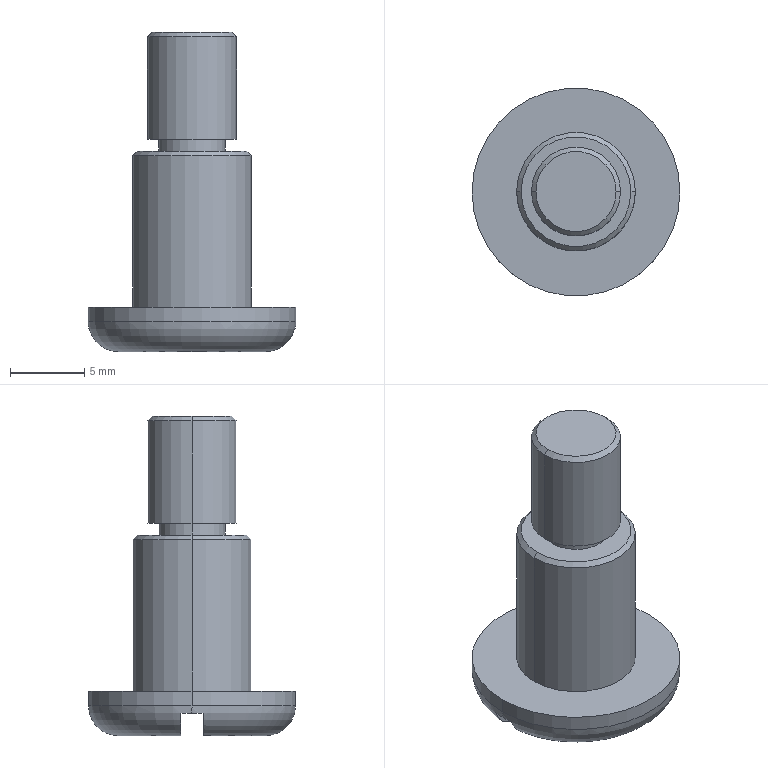Part | SolidWorks | features ICE 4, Chamfer 1, Extrusion 1, Fillet 1 | 1 solid | 23 faces | box 14 x 14 x 21.5 mm | volume 1140 mm3 | plane 9 | cylinder 8 | cone 4 | torus 2 | commonest cylinder face diameters 4.5 x2 6 x2 8 x2 14 x2
STEP:
#1=CARTESIAN_POINT('',(2.7,0.,21.5));
#2=VERTEX_POINT('',#1);
#3=CARTESIAN_POINT('',(-2.7,0.,21.5));
#4=VERTEX_POINT('',#3);
#5=CARTESIAN_POINT('',(0.,0.,21.5));
#6=DIRECTION('',(0.,0.,1.));
#7=DIRECTION('',(1.,0.,0.));
#8=AXIS2_PLACEMENT_3D('',#5,#6,#7);
#9=CIRCLE('',#8,2.7);
#10=EDGE_CURVE('',#2,#4,#9,.T.);
#11=ORIENTED_EDGE('',*,*,#10,.F.);
#12=CARTESIAN_POINT('',(3.,0.,21.2));
#13=VERTEX_POINT('',#12);
#14=CARTESIAN_POINT('',(2.7,0.,21.5));
#15=DIRECTION('',(0.7071,0.,-0.7071));
#16=VECTOR('',#15,1000.);
#17=LINE('',#14,#16);
#18=EDGE_CURVE('',#2,#13,#17,.T.);
#19=ORIENTED_EDGE('',*,*,#18,.T.);
#20=CARTESIAN_POINT('',(-3.,0.,21.2));
#21=VERTEX_POINT('',#20);
#22=CARTESIAN_POINT('',(0.,0.,21.2));
#23=DIRECTION('',(0.,0.,-1.));
#24=DIRECTION('',(1.,0.,0.));
#25=AXIS2_PLACEMENT_3D('',#22,#23,#24);
#26=CIRCLE('',#25,3.);
#27=EDGE_CURVE('',#21,#13,#26,.T.);
#28=ORIENTED_EDGE('',*,*,#27,.F.);
#29=CARTESIAN_POINT('',(-2.7,0.,21.5));
#30=DIRECTION('',(-0.7071,0.,-0.7071));
#31=VECTOR('',#30,1000.);
#32=LINE('',#29,#31);
#33=EDGE_CURVE('',#4,#21,#32,.T.);
#34=ORIENTED_EDGE('',*,*,#33,.F.);
#35=EDGE_LOOP('',(#11,#19,#28,#34));
#36=FACE_OUTER_BOUND('',#35,.T.);
#37=CARTESIAN_POINT('',(0.,0.,21.5));
#38=DIRECTION('',(0.,0.,-1.));
#39=DIRECTION('',(-1.,0.,0.));
#40=AXIS2_PLACEMENT_3D('',#37,#38,#39);
#41=CONICAL_SURFACE('',#40,2.7,0.7854);
#42=ADVANCED_FACE('',(#36),#41,.T.);
#43=CARTESIAN_POINT('',(3.7,0.,13.5));
#44=VERTEX_POINT('',#43);
#45=CARTESIAN_POINT('',(-3.7,0.,13.5));
#46=VERTEX_POINT('',#45);
#47=CARTESIAN_POINT('',(0.,0.,13.5));
#48=DIRECTION('',(0.,0.,1.));
#49=DIRECTION('',(1.,0.,0.));
#50=AXIS2_PLACEMENT_3D('',#47,#48,#49);
#51=CIRCLE('',#50,3.7);
#52=EDGE_CURVE('',#44,#46,#51,.T.);
#53=ORIENTED_EDGE('',*,*,#52,.F.);
#54=CARTESIAN_POINT('',(4.,0.,13.2));
#55=VERTEX_POINT('',#54);
#56=CARTESIAN_POINT('',(3.7,0.,13.5));
#57=DIRECTION('',(0.7071,0.,-0.7071));
#58=VECTOR('',#57,1000.);
#59=LINE('',#56,#58);
#60=EDGE_CURVE('',#44,#55,#59,.T.);
#61=ORIENTED_EDGE('',*,*,#60,.T.);
#62=CARTESIAN_POINT('',(-4.,0.,13.2));
#63=VERTEX_POINT('',#62);
#64=CARTESIAN_POINT('',(0.,0.,13.2));
#65=DIRECTION('',(0.,0.,-1.));
#66=DIRECTION('',(1.,0.,0.));
#67=AXIS2_PLACEMENT_3D('',#64,#65,#66);
#68=CIRCLE('',#67,4.);
#69=EDGE_CURVE('',#63,#55,#68,.T.);
#70=ORIENTED_EDGE('',*,*,#69,.F.);
#71=CARTESIAN_POINT('',(-3.7,0.,13.5));
#72=DIRECTION('',(-0.7071,0.,-0.7071));
#73=VECTOR('',#72,1000.);
#74=LINE('',#71,#73);
#75=EDGE_CURVE('',#46,#63,#74,.T.);
#76=ORIENTED_EDGE('',*,*,#75,.F.);
#77=EDGE_LOOP('',(#53,#61,#70,#76));
#78=FACE_OUTER_BOUND('',#77,.T.);
#79=CARTESIAN_POINT('',(0.,0.,13.5));
#80=DIRECTION('',(0.,0.,-1.));
#81=DIRECTION('',(-1.,0.,0.));
#82=AXIS2_PLACEMENT_3D('',#79,#80,#81);
#83=CONICAL_SURFACE('',#82,3.7,0.7854);
#84=ADVANCED_FACE('',(#78),#83,.T.);
#85=CARTESIAN_POINT('',(-6.936,0.,1.5));
#86=VERTEX_POINT('',#85);
#87=CARTESIAN_POINT('',(-6.896,0.75,1.5));
#88=VERTEX_POINT('',#87);
#89=CARTESIAN_POINT('',(0.,0.,1.5));
#90=DIRECTION('',(0.,0.,-1.));
#91=DIRECTION('',(1.,0.,0.));
#92=AXIS2_PLACEMENT_3D('',#89,#90,#91);
#93=CIRCLE('',#92,6.936);
#94=EDGE_CURVE('',#86,#88,#93,.T.);
#95=ORIENTED_EDGE('',*,*,#94,.F.);
#96=CARTESIAN_POINT('',(-7.,0.,2.));
#97=VERTEX_POINT('',#96);
#98=CARTESIAN_POINT('',(-5.,0.,2.));
#99=DIRECTION('',(0.,1.,0.));
#100=DIRECTION('',(-1.,0.,0.));
#101=AXIS2_PLACEMENT_3D('',#98,#99,#100);
#102=CIRCLE('',#101,2.);
#103=EDGE_CURVE('',#86,#97,#102,.T.);
#104=ORIENTED_EDGE('',*,*,#103,.T.);
#105=CARTESIAN_POINT('',(7.,0.,2.));
#106=VERTEX_POINT('',#105);
#107=CARTESIAN_POINT('',(0.,0.,2.));
#108=DIRECTION('',(0.,0.,1.));
#109=DIRECTION('',(1.,0.,0.));
#110=AXIS2_PLACEMENT_3D('',#107,#108,#109);
#111=CIRCLE('',#110,7.);
#112=EDGE_CURVE('',#106,#97,#111,.T.);
#113=ORIENTED_EDGE('',*,*,#112,.F.);
#114=CARTESIAN_POINT('',(6.936,0.,1.5));
#115=VERTEX_POINT('',#114);
#116=CARTESIAN_POINT('',(5.,0.,2.));
#117=DIRECTION('',(0.,-1.,0.));
#118=DIRECTION('',(0.,0.,-1.));
#119=AXIS2_PLACEMENT_3D('',#116,#117,#118);
#120=CIRCLE('',#119,2.);
#121=EDGE_CURVE('',#115,#106,#120,.T.);
#122=ORIENTED_EDGE('',*,*,#121,.F.);
#123=CARTESIAN_POINT('',(6.896,0.75,1.5));
#124=VERTEX_POINT('',#123);
#125=CARTESIAN_POINT('',(0.,0.,1.5));
#126=DIRECTION('',(0.,0.,-1.));
#127=DIRECTION('',(1.,0.,0.));
#128=AXIS2_PLACEMENT_3D('',#125,#126,#127);
#129=CIRCLE('',#128,6.936);
#130=EDGE_CURVE('',#124,#115,#129,.T.);
#131=ORIENTED_EDGE('',*,*,#130,.F.);
#132=CARTESIAN_POINT('',(4.943,0.75,0.));
#133=VERTEX_POINT('',#132);
#134=CARTESIAN_POINT('',(4.943,0.75,0.));
#135=CARTESIAN_POINT('',(5.165,0.75,0.));
#136=CARTESIAN_POINT('',(5.384,0.75,0.03577));
#137=CARTESIAN_POINT('',(5.804,0.75,0.1774));
#138=CARTESIAN_POINT('',(6.,0.75,0.2814));
#139=CARTESIAN_POINT('',(6.353,0.75,0.5514));
#140=CARTESIAN_POINT('',(6.504,0.75,0.7128));
#141=CARTESIAN_POINT('',(6.75,0.75,1.083));
#142=CARTESIAN_POINT('',(6.84,0.75,1.285));
#143=CARTESIAN_POINT('',(6.896,0.75,1.5));
#144=B_SPLINE_CURVE_WITH_KNOTS('',3,(#134,#135,#136,#137,#138,#139,#140,#141,#142,#143),.UNSPECIFIED.,.F.,.F.,(4,2,2,2,4),(0.002167,0.002826,0.003486,0.004145,0.004804),.UNSPECIFIED.);
#145=EDGE_CURVE('',#133,#124,#144,.T.);
#146=ORIENTED_EDGE('',*,*,#145,.F.);
#147=CARTESIAN_POINT('',(-4.943,0.75,0.));
#148=VERTEX_POINT('',#147);
#149=CARTESIAN_POINT('',(0.,0.,0.));
#150=DIRECTION('',(0.,0.,-1.));
#151=DIRECTION('',(1.,0.,0.));
#152=AXIS2_PLACEMENT_3D('',#149,#150,#151);
#153=CIRCLE('',#152,5.);
#154=EDGE_CURVE('',#148,#133,#153,.T.);
#155=ORIENTED_EDGE('',*,*,#154,.F.);
#156=CARTESIAN_POINT('',(-6.896,0.75,1.5));
#157=CARTESIAN_POINT('',(-6.84,0.75,1.285));
#158=CARTESIAN_POINT('',(-6.75,0.75,1.083));
#159=CARTESIAN_POINT('',(-6.505,0.75,0.7142));
#160=CARTESIAN_POINT('',(-6.35,0.75,0.549));
#161=CARTESIAN_POINT('',(-6.087,0.75,0.3486));
#162=CARTESIAN_POINT('',(-5.995,0.75,0.2893));
#163=CARTESIAN_POINT('',(-5.801,0.75,0.1858));
#164=CARTESIAN_POINT('',(-5.698,0.75,0.1415));
#165=CARTESIAN_POINT('',(-5.489,0.75,0.07119));
#166=CARTESIAN_POINT('',(-5.383,0.75,0.04473));
#167=CARTESIAN_POINT('',(-5.165,0.75,0.009087));
#168=CARTESIAN_POINT('',(-5.054,0.75,0.));
#169=CARTESIAN_POINT('',(-4.943,0.75,0.));
#170=B_SPLINE_CURVE_WITH_KNOTS('',3,(#156,#157,#158,#159,#160,#161,#162,#163,#164,#165,#166,#167,#168,#169),.UNSPECIFIED.,.F.,.F.,(4,2,2,2,2,2,4),(0.01146,0.01212,0.01278,0.0131,0.01343,0.01376,0.01409),.UNSPECIFIED.);
#171=EDGE_CURVE('',#88,#148,#170,.T.);
#172=ORIENTED_EDGE('',*,*,#171,.F.);
#173=EDGE_LOOP('',(#95,#104,#113,#122,#131,#146,#155,#172));
#174=FACE_OUTER_BOUND('',#173,.T.);
#175=CARTESIAN_POINT('',(0.,0.,2.));
#176=DIRECTION('',(0.,0.,1.));
#177=DIRECTION('',(1.,0.,0.));
#178=AXIS2_PLACEMENT_3D('',#175,#176,#177);
#179=TOROIDAL_SURFACE('',#178,5.,2.);
#180=ADVANCED_FACE('',(#174),#179,.T.);
#181=ORIENTED_EDGE('',*,*,#27,.T.);
#182=CARTESIAN_POINT('',(3.,0.,14.3));
#183=VERTEX_POINT('',#182);
#184=CARTESIAN_POINT('',(3.,0.,21.5));
#185=DIRECTION('',(0.,0.,-1.));
#186=VECTOR('',#185,1000.);
#187=LINE('',#184,#186);
#188=EDGE_CURVE('',#13,#183,#187,.T.);
#189=ORIENTED_EDGE('',*,*,#188,.T.);
#190=CARTESIAN_POINT('',(-3.,0.,14.3));
#191=VERTEX_POINT('',#190);
#192=CARTESIAN_POINT('',(0.,0.,14.3));
#193=DIRECTION('',(0.,0.,1.));
#194=DIRECTION('',(1.,0.,0.));
#195=AXIS2_PLACEMENT_3D('',#192,#193,#194);
#196=CIRCLE('',#195,3.);
#197=EDGE_CURVE('',#183,#191,#196,.T.);
#198=ORIENTED_EDGE('',*,*,#197,.T.);
#199=CARTESIAN_POINT('',(-3.,0.,21.5));
#200=DIRECTION('',(0.,0.,-1.));
#201=VECTOR('',#200,1000.);
#202=LINE('',#199,#201);
#203=EDGE_CURVE('',#21,#191,#202,.T.);
#204=ORIENTED_EDGE('',*,*,#203,.F.);
#205=EDGE_LOOP('',(#181,#189,#198,#204));
#206=FACE_OUTER_BOUND('',#205,.T.);
#207=CARTESIAN_POINT('',(0.,0.,21.5));
#208=DIRECTION('',(0.,0.,-1.));
#209=DIRECTION('',(-1.,0.,0.));
#210=AXIS2_PLACEMENT_3D('',#207,#208,#209);
#211=CYLINDRICAL_SURFACE('',#210,3.);
#212=ADVANCED_FACE('',(#206),#211,.T.);
#213=CARTESIAN_POINT('',(2.25,0.,14.3));
#214=VERTEX_POINT('',#213);
#215=CARTESIAN_POINT('',(-2.25,0.,14.3));
#216=VERTEX_POINT('',#215);
#217=CARTESIAN_POINT('',(0.,0.,14.3));
#218=DIRECTION('',(0.,0.,1.));
#219=DIRECTION('',(1.,0.,0.));
#220=AXIS2_PLACEMENT_3D('',#217,#218,#219);
#221=CIRCLE('',#220,2.25);
#222=EDGE_CURVE('',#214,#216,#221,.T.);
#223=ORIENTED_EDGE('',*,*,#222,.F.);
#224=CARTESIAN_POINT('',(2.25,0.,13.5));
#225=VERTEX_POINT('',#224);
#226=CARTESIAN_POINT('',(2.25,0.,14.3));
#227=DIRECTION('',(0.,0.,-1.));
#228=VECTOR('',#227,1000.);
#229=LINE('',#226,#228);
#230=EDGE_CURVE('',#214,#225,#229,.T.);
#231=ORIENTED_EDGE('',*,*,#230,.T.);
#232=CARTESIAN_POINT('',(-2.25,0.,13.5));
#233=VERTEX_POINT('',#232);
#234=CARTESIAN_POINT('',(0.,0.,13.5));
#235=DIRECTION('',(0.,0.,1.));
#236=DIRECTION('',(1.,0.,0.));
#237=AXIS2_PLACEMENT_3D('',#234,#235,#236);
#238=CIRCLE('',#237,2.25);
#239=EDGE_CURVE('',#225,#233,#238,.T.);
#240=ORIENTED_EDGE('',*,*,#239,.T.);
#241=CARTESIAN_POINT('',(-2.25,0.,14.3));
#242=DIRECTION('',(0.,0.,-1.));
#243=VECTOR('',#242,1000.);
#244=LINE('',#241,#243);
#245=EDGE_CURVE('',#216,#233,#244,.T.);
#246=ORIENTED_EDGE('',*,*,#245,.F.);
#247=EDGE_LOOP('',(#223,#231,#240,#246));
#248=FACE_OUTER_BOUND('',#247,.T.);
#249=CARTESIAN_POINT('',(0.,0.,14.3));
#250=DIRECTION('',(0.,0.,-1.));
#251=DIRECTION('',(-1.,0.,0.));
#252=AXIS2_PLACEMENT_3D('',#249,#250,#251);
#253=CYLINDRICAL_SURFACE('',#252,2.25);
#254=ADVANCED_FACE('',(#248),#253,.T.);
#255=ORIENTED_EDGE('',*,*,#69,.T.);
#256=CARTESIAN_POINT('',(4.,0.,3.));
#257=VERTEX_POINT('',#256);
#258=CARTESIAN_POINT('',(4.,0.,13.5));
#259=DIRECTION('',(0.,0.,-1.));
#260=VECTOR('',#259,1000.);
#261=LINE('',#258,#260);
#262=EDGE_CURVE('',#55,#257,#261,.T.);
#263=ORIENTED_EDGE('',*,*,#262,.T.);
#264=CARTESIAN_POINT('',(-4.,0.,3.));
#265=VERTEX_POINT('',#264);
#266=CARTESIAN_POINT('',(0.,0.,3.));
#267=DIRECTION('',(0.,0.,1.));
#268=DIRECTION('',(1.,0.,0.));
#269=AXIS2_PLACEMENT_3D('',#266,#267,#268);
#270=CIRCLE('',#269,4.);
#271=EDGE_CURVE('',#257,#265,#270,.T.);
#272=ORIENTED_EDGE('',*,*,#271,.T.);
#273=CARTESIAN_POINT('',(-4.,0.,13.5));
#274=DIRECTION('',(0.,0.,-1.));
#275=VECTOR('',#274,1000.);
#276=LINE('',#273,#275);
#277=EDGE_CURVE('',#63,#265,#276,.T.);
#278=ORIENTED_EDGE('',*,*,#277,.F.);
#279=EDGE_LOOP('',(#255,#263,#272,#278));
#280=FACE_OUTER_BOUND('',#279,.T.);
#281=CARTESIAN_POINT('',(0.,0.,13.5));
#282=DIRECTION('',(0.,0.,-1.));
#283=DIRECTION('',(-1.,0.,0.));
#284=AXIS2_PLACEMENT_3D('',#281,#282,#283);
#285=CYLINDRICAL_SURFACE('',#284,4.);
#286=ADVANCED_FACE('',(#280),#285,.T.);
#287=CARTESIAN_POINT('',(7.,0.,3.));
#288=VERTEX_POINT('',#287);
#289=CARTESIAN_POINT('',(-7.,0.,3.));
#290=VERTEX_POINT('',#289);
#291=CARTESIAN_POINT('',(0.,0.,3.));
#292=DIRECTION('',(0.,0.,1.));
#293=DIRECTION('',(1.,0.,0.));
#294=AXIS2_PLACEMENT_3D('',#291,#292,#293);
#295=CIRCLE('',#294,7.);
#296=EDGE_CURVE('',#288,#290,#295,.T.);
#297=ORIENTED_EDGE('',*,*,#296,.F.);
#298=CARTESIAN_POINT('',(7.,0.,3.));
#299=DIRECTION('',(0.,0.,-1.));
#300=VECTOR('',#299,1000.);
#301=LINE('',#298,#300);
#302=EDGE_CURVE('',#288,#106,#301,.T.);
#303=ORIENTED_EDGE('',*,*,#302,.T.);
#304=ORIENTED_EDGE('',*,*,#112,.T.);
#305=CARTESIAN_POINT('',(-7.,0.,3.));
#306=DIRECTION('',(0.,0.,-1.));
#307=VECTOR('',#306,1000.);
#308=LINE('',#305,#307);
#309=EDGE_CURVE('',#290,#97,#308,.T.);
#310=ORIENTED_EDGE('',*,*,#309,.F.);
#311=EDGE_LOOP('',(#297,#303,#304,#310));
#312=FACE_OUTER_BOUND('',#311,.T.);
#313=CARTESIAN_POINT('',(0.,0.,3.));
#314=DIRECTION('',(0.,0.,-1.));
#315=DIRECTION('',(-1.,0.,0.));
#316=AXIS2_PLACEMENT_3D('',#313,#314,#315);
#317=CYLINDRICAL_SURFACE('',#316,7.);
#318=ADVANCED_FACE('',(#312),#317,.T.);
#319=CARTESIAN_POINT('',(4.943,-0.75,0.));
#320=VERTEX_POINT('',#319);
#321=CARTESIAN_POINT('',(-4.943,-0.75,0.));
#322=VERTEX_POINT('',#321);
#323=CARTESIAN_POINT('',(0.,0.,0.));
#324=DIRECTION('',(0.,0.,-1.));
#325=DIRECTION('',(1.,0.,0.));
#326=AXIS2_PLACEMENT_3D('',#323,#324,#325);
#327=CIRCLE('',#326,5.);
#328=EDGE_CURVE('',#320,#322,#327,.T.);
#329=ORIENTED_EDGE('',*,*,#328,.T.);
#330=CARTESIAN_POINT('',(8.518,-0.75,0.));
#331=DIRECTION('',(-1.,0.,0.));
#332=VECTOR('',#331,1000.);
#333=LINE('',#330,#332);
#334=EDGE_CURVE('',#320,#322,#333,.T.);
#335=ORIENTED_EDGE('',*,*,#334,.F.);
#336=EDGE_LOOP('',(#329,#335));
#337=FACE_OUTER_BOUND('',#336,.T.);
#338=CARTESIAN_POINT('',(0.,0.,0.));
#339=DIRECTION('',(0.,0.,1.));
#340=DIRECTION('',(1.,0.,0.));
#341=AXIS2_PLACEMENT_3D('',#338,#339,#340);
#342=PLANE('',#341);
#343=ADVANCED_FACE('',(#337),#342,.F.);
#344=ORIENTED_EDGE('',*,*,#302,.F.);
#345=CARTESIAN_POINT('',(0.,0.,3.));
#346=DIRECTION('',(0.,0.,1.));
#347=DIRECTION('',(1.,0.,0.));
#348=AXIS2_PLACEMENT_3D('',#345,#346,#347);
#349=CIRCLE('',#348,7.);
#350=EDGE_CURVE('',#290,#288,#349,.T.);
#351=ORIENTED_EDGE('',*,*,#350,.F.);
#352=ORIENTED_EDGE('',*,*,#309,.T.);
#353=CARTESIAN_POINT('',(0.,0.,2.));
#354=DIRECTION('',(0.,0.,1.));
#355=DIRECTION('',(1.,0.,0.));
#356=AXIS2_PLACEMENT_3D('',#353,#354,#355);
#357=CIRCLE('',#356,7.);
#358=EDGE_CURVE('',#97,#106,#357,.T.);
#359=ORIENTED_EDGE('',*,*,#358,.T.);
#360=EDGE_LOOP('',(#344,#351,#352,#359));
#361=FACE_OUTER_BOUND('',#360,.T.);
#362=CARTESIAN_POINT('',(0.,0.,3.));
#363=DIRECTION('',(0.,0.,-1.));
#364=DIRECTION('',(-1.,0.,0.));
#365=AXIS2_PLACEMENT_3D('',#362,#363,#364);
#366=CYLINDRICAL_SURFACE('',#365,7.);
#367=ADVANCED_FACE('',(#361),#366,.T.);
#368=CARTESIAN_POINT('',(0.,0.,3.));
#369=DIRECTION('',(0.,0.,1.));
#370=DIRECTION('',(1.,0.,0.));
#371=AXIS2_PLACEMENT_3D('',#368,#369,#370);
#372=CIRCLE('',#371,4.);
#373=EDGE_CURVE('',#265,#257,#372,.T.);
#374=ORIENTED_EDGE('',*,*,#373,.F.);
#375=ORIENTED_EDGE('',*,*,#271,.F.);
#376=EDGE_LOOP('',(#374,#375));
#377=FACE_BOUND('',#376,.T.);
#378=ORIENTED_EDGE('',*,*,#350,.T.);
#379=ORIENTED_EDGE('',*,*,#296,.T.);
#380=EDGE_LOOP('',(#378,#379));
#381=FACE_OUTER_BOUND('',#380,.T.);
#382=CARTESIAN_POINT('',(0.,0.,3.));
#383=DIRECTION('',(0.,0.,1.));
#384=DIRECTION('',(1.,0.,0.));
#385=AXIS2_PLACEMENT_3D('',#382,#383,#384);
#386=PLANE('',#385);
#387=ADVANCED_FACE('',(#377,#381),#386,.T.);
#388=ORIENTED_EDGE('',*,*,#154,.T.);
#389=CARTESIAN_POINT('',(8.518,0.75,0.));
#390=DIRECTION('',(1.,0.,0.));
#391=VECTOR('',#390,1000.);
#392=LINE('',#389,#391);
#393=EDGE_CURVE('',#148,#133,#392,.T.);
#394=ORIENTED_EDGE('',*,*,#393,.F.);
#395=EDGE_LOOP('',(#388,#394));
#396=FACE_OUTER_BOUND('',#395,.T.);
#397=CARTESIAN_POINT('',(0.,0.,0.));
#398=DIRECTION('',(0.,0.,1.));
#399=DIRECTION('',(1.,0.,0.));
#400=AXIS2_PLACEMENT_3D('',#397,#398,#399);
#401=PLANE('',#400);
#402=ADVANCED_FACE('',(#396),#401,.F.);
#403=ORIENTED_EDGE('',*,*,#262,.F.);
#404=CARTESIAN_POINT('',(0.,0.,13.2));
#405=DIRECTION('',(0.,0.,-1.));
#406=DIRECTION('',(1.,0.,0.));
#407=AXIS2_PLACEMENT_3D('',#404,#405,#406);
#408=CIRCLE('',#407,4.);
#409=EDGE_CURVE('',#55,#63,#408,.T.);
#410=ORIENTED_EDGE('',*,*,#409,.T.);
#411=ORIENTED_EDGE('',*,*,#277,.T.);
#412=ORIENTED_EDGE('',*,*,#373,.T.);
#413=EDGE_LOOP('',(#403,#410,#411,#412));
#414=FACE_OUTER_BOUND('',#413,.T.);
#415=CARTESIAN_POINT('',(0.,0.,13.5));
#416=DIRECTION('',(0.,0.,-1.));
#417=DIRECTION('',(-1.,0.,0.));
#418=AXIS2_PLACEMENT_3D('',#415,#416,#417);
#419=CYLINDRICAL_SURFACE('',#418,4.);
#420=ADVANCED_FACE('',(#414),#419,.T.);
#421=CARTESIAN_POINT('',(0.,0.,13.5));
#422=DIRECTION('',(0.,0.,1.));
#423=DIRECTION('',(1.,0.,0.));
#424=AXIS2_PLACEMENT_3D('',#421,#422,#423);
#425=CIRCLE('',#424,3.7);
#426=EDGE_CURVE('',#46,#44,#425,.T.);
#427=ORIENTED_EDGE('',*,*,#426,.T.);
#428=ORIENTED_EDGE('',*,*,#52,.T.);
#429=EDGE_LOOP('',(#427,#428));
#430=FACE_OUTER_BOUND('',#429,.T.);
#431=CARTESIAN_POINT('',(0.,0.,13.5));
#432=DIRECTION('',(0.,0.,1.));
#433=DIRECTION('',(1.,0.,0.));
#434=AXIS2_PLACEMENT_3D('',#431,#432,#433);
#435=CIRCLE('',#434,2.25);
#436=EDGE_CURVE('',#233,#225,#435,.T.);
#437=ORIENTED_EDGE('',*,*,#436,.F.);
#438=ORIENTED_EDGE('',*,*,#239,.F.);
#439=EDGE_LOOP('',(#437,#438));
#440=FACE_BOUND('',#439,.T.);
#441=CARTESIAN_POINT('',(0.,0.,13.5));
#442=DIRECTION('',(0.,0.,1.));
#443=DIRECTION('',(1.,0.,0.));
#444=AXIS2_PLACEMENT_3D('',#441,#442,#443);
#445=PLANE('',#444);
#446=ADVANCED_FACE('',(#430,#440),#445,.T.);
#447=CARTESIAN_POINT('',(0.,0.,14.3));
#448=DIRECTION('',(0.,0.,1.));
#449=DIRECTION('',(1.,0.,0.));
#450=AXIS2_PLACEMENT_3D('',#447,#448,#449);
#451=CIRCLE('',#450,3.);
#452=EDGE_CURVE('',#191,#183,#451,.T.);
#453=ORIENTED_EDGE('',*,*,#452,.F.);
#454=ORIENTED_EDGE('',*,*,#197,.F.);
#455=EDGE_LOOP('',(#453,#454));
#456=FACE_OUTER_BOUND('',#455,.T.);
#457=CARTESIAN_POINT('',(0.,0.,14.3));
#458=DIRECTION('',(0.,0.,1.));
#459=DIRECTION('',(1.,0.,0.));
#460=AXIS2_PLACEMENT_3D('',#457,#458,#459);
#461=CIRCLE('',#460,2.25);
#462=EDGE_CURVE('',#216,#214,#461,.T.);
#463=ORIENTED_EDGE('',*,*,#462,.T.);
#464=ORIENTED_EDGE('',*,*,#222,.T.);
#465=EDGE_LOOP('',(#463,#464));
#466=FACE_BOUND('',#465,.T.);
#467=CARTESIAN_POINT('',(0.,0.,14.3));
#468=DIRECTION('',(0.,0.,1.));
#469=DIRECTION('',(1.,0.,0.));
#470=AXIS2_PLACEMENT_3D('',#467,#468,#469);
#471=PLANE('',#470);
#472=ADVANCED_FACE('',(#456,#466),#471,.F.);
#473=ORIENTED_EDGE('',*,*,#230,.F.);
#474=ORIENTED_EDGE('',*,*,#462,.F.);
#475=ORIENTED_EDGE('',*,*,#245,.T.);
#476=ORIENTED_EDGE('',*,*,#436,.T.);
#477=EDGE_LOOP('',(#473,#474,#475,#476));
#478=FACE_OUTER_BOUND('',#477,.T.);
#479=CARTESIAN_POINT('',(0.,0.,14.3));
#480=DIRECTION('',(0.,0.,-1.));
#481=DIRECTION('',(-1.,0.,0.));
#482=AXIS2_PLACEMENT_3D('',#479,#480,#481);
#483=CYLINDRICAL_SURFACE('',#482,2.25);
#484=ADVANCED_FACE('',(#478),#483,.T.);
#485=CARTESIAN_POINT('',(0.,0.,21.5));
#486=DIRECTION('',(0.,0.,1.));
#487=DIRECTION('',(1.,0.,0.));
#488=AXIS2_PLACEMENT_3D('',#485,#486,#487);
#489=CIRCLE('',#488,2.7);
#490=EDGE_CURVE('',#4,#2,#489,.T.);
#491=ORIENTED_EDGE('',*,*,#490,.T.);
#492=ORIENTED_EDGE('',*,*,#10,.T.);
#493=EDGE_LOOP('',(#491,#492));
#494=FACE_OUTER_BOUND('',#493,.T.);
#495=CARTESIAN_POINT('',(0.,0.,21.5));
#496=DIRECTION('',(0.,0.,1.));
#497=DIRECTION('',(1.,0.,0.));
#498=AXIS2_PLACEMENT_3D('',#495,#496,#497);
#499=PLANE('',#498);
#500=ADVANCED_FACE('',(#494),#499,.T.);
#501=ORIENTED_EDGE('',*,*,#188,.F.);
#502=CARTESIAN_POINT('',(0.,0.,21.2));
#503=DIRECTION('',(0.,0.,-1.));
#504=DIRECTION('',(1.,0.,0.));
#505=AXIS2_PLACEMENT_3D('',#502,#503,#504);
#506=CIRCLE('',#505,3.);
#507=EDGE_CURVE('',#13,#21,#506,.T.);
#508=ORIENTED_EDGE('',*,*,#507,.T.);
#509=ORIENTED_EDGE('',*,*,#203,.T.);
#510=ORIENTED_EDGE('',*,*,#452,.T.);
#511=EDGE_LOOP('',(#501,#508,#509,#510));
#512=FACE_OUTER_BOUND('',#511,.T.);
#513=CARTESIAN_POINT('',(0.,0.,21.5));
#514=DIRECTION('',(0.,0.,-1.));
#515=DIRECTION('',(-1.,0.,0.));
#516=AXIS2_PLACEMENT_3D('',#513,#514,#515);
#517=CYLINDRICAL_SURFACE('',#516,3.);
#518=ADVANCED_FACE('',(#512),#517,.T.);
#519=ORIENTED_EDGE('',*,*,#103,.F.);
#520=CARTESIAN_POINT('',(-6.896,-0.75,1.5));
#521=VERTEX_POINT('',#520);
#522=CARTESIAN_POINT('',(0.,0.,1.5));
#523=DIRECTION('',(0.,0.,-1.));
#524=DIRECTION('',(1.,0.,0.));
#525=AXIS2_PLACEMENT_3D('',#522,#523,#524);
#526=CIRCLE('',#525,6.936);
#527=EDGE_CURVE('',#521,#86,#526,.T.);
#528=ORIENTED_EDGE('',*,*,#527,.F.);
#529=CARTESIAN_POINT('',(-4.943,-0.75,0.));
#530=CARTESIAN_POINT('',(-5.163,-0.75,0.));
#531=CARTESIAN_POINT('',(-5.386,-0.75,0.03632));
#532=CARTESIAN_POINT('',(-5.802,-0.75,0.1767));
#533=CARTESIAN_POINT('',(-6.001,-0.75,0.2819));
#534=CARTESIAN_POINT('',(-6.352,-0.75,0.5513));
#535=CARTESIAN_POINT('',(-6.505,-0.75,0.7149));
#536=CARTESIAN_POINT('',(-6.688,-0.75,0.99));
#537=CARTESIAN_POINT('',(-6.742,-0.75,1.088));
#538=CARTESIAN_POINT('',(-6.832,-0.75,1.29));
#539=CARTESIAN_POINT('',(-6.868,-0.75,1.394));
#540=CARTESIAN_POINT('',(-6.896,-0.75,1.5));
#541=B_SPLINE_CURVE_WITH_KNOTS('',3,(#529,#530,#531,#532,#533,#534,#535,#536,#537,#538,#539,#540),.UNSPECIFIED.,.F.,.F.,(4,2,2,2,2,4),(0.01108,0.01174,0.0124,0.01306,0.01339,0.01372),.UNSPECIFIED.);
#542=EDGE_CURVE('',#322,#521,#541,.T.);
#543=ORIENTED_EDGE('',*,*,#542,.F.);
#544=ORIENTED_EDGE('',*,*,#328,.F.);
#545=CARTESIAN_POINT('',(6.896,-0.75,1.5));
#546=VERTEX_POINT('',#545);
#547=CARTESIAN_POINT('',(6.896,-0.75,1.5));
#548=CARTESIAN_POINT('',(6.841,-0.75,1.287));
#549=CARTESIAN_POINT('',(6.748,-0.75,1.081));
#550=CARTESIAN_POINT('',(6.505,-0.75,0.715));
#551=CARTESIAN_POINT('',(6.351,-0.75,0.5501));
#552=CARTESIAN_POINT('',(6.002,-0.75,0.2829));
#553=CARTESIAN_POINT('',(5.802,-0.75,0.1768));
#554=CARTESIAN_POINT('',(5.386,-0.75,0.03638));
#555=CARTESIAN_POINT('',(5.163,-0.75,0.));
#556=CARTESIAN_POINT('',(4.943,-0.75,0.));
#557=B_SPLINE_CURVE_WITH_KNOTS('',3,(#547,#548,#549,#550,#551,#552,#553,#554,#555,#556),.UNSPECIFIED.,.F.,.F.,(4,2,2,2,4),(0.007787,0.008446,0.009106,0.009765,0.01042),.UNSPECIFIED.);
#558=EDGE_CURVE('',#546,#320,#557,.T.);
#559=ORIENTED_EDGE('',*,*,#558,.F.);
#560=CARTESIAN_POINT('',(0.,0.,1.5));
#561=DIRECTION('',(0.,0.,-1.));
#562=DIRECTION('',(1.,0.,0.));
#563=AXIS2_PLACEMENT_3D('',#560,#561,#562);
#564=CIRCLE('',#563,6.936);
#565=EDGE_CURVE('',#115,#546,#564,.T.);
#566=ORIENTED_EDGE('',*,*,#565,.F.);
#567=ORIENTED_EDGE('',*,*,#121,.T.);
#568=ORIENTED_EDGE('',*,*,#358,.F.);
#569=EDGE_LOOP('',(#519,#528,#543,#544,#559,#566,#567,#568));
#570=FACE_OUTER_BOUND('',#569,.T.);
#571=CARTESIAN_POINT('',(0.,0.,2.));
#572=DIRECTION('',(0.,0.,1.));
#573=DIRECTION('',(1.,0.,0.));
#574=AXIS2_PLACEMENT_3D('',#571,#572,#573);
#575=TOROIDAL_SURFACE('',#574,5.,2.);
#576=ADVANCED_FACE('',(#570),#575,.T.);
#577=ORIENTED_EDGE('',*,*,#542,.T.);
#578=CARTESIAN_POINT('',(8.518,-0.75,1.5));
#579=DIRECTION('',(-1.,0.,0.));
#580=VECTOR('',#579,1000.);
#581=LINE('',#578,#580);
#582=EDGE_CURVE('',#546,#521,#581,.T.);
#583=ORIENTED_EDGE('',*,*,#582,.F.);
#584=ORIENTED_EDGE('',*,*,#558,.T.);
#585=ORIENTED_EDGE('',*,*,#334,.T.);
#586=EDGE_LOOP('',(#577,#583,#584,#585));
#587=FACE_OUTER_BOUND('',#586,.T.);
#588=CARTESIAN_POINT('',(8.518,-0.75,1.5));
#589=DIRECTION('',(0.,-1.,0.));
#590=DIRECTION('',(0.,0.,-1.));
#591=AXIS2_PLACEMENT_3D('',#588,#589,#590);
#592=PLANE('',#591);
#593=ADVANCED_FACE('',(#587),#592,.F.);
#594=ORIENTED_EDGE('',*,*,#171,.T.);
#595=ORIENTED_EDGE('',*,*,#393,.T.);
#596=ORIENTED_EDGE('',*,*,#145,.T.);
#597=CARTESIAN_POINT('',(8.518,0.75,1.5));
#598=DIRECTION('',(1.,0.,0.));
#599=VECTOR('',#598,1000.);
#600=LINE('',#597,#599);
#601=EDGE_CURVE('',#88,#124,#600,.T.);
#602=ORIENTED_EDGE('',*,*,#601,.F.);
#603=EDGE_LOOP('',(#594,#595,#596,#602));
#604=FACE_OUTER_BOUND('',#603,.T.);
#605=CARTESIAN_POINT('',(8.518,0.75,1.5));
#606=DIRECTION('',(0.,1.,0.));
#607=DIRECTION('',(0.,0.,1.));
#608=AXIS2_PLACEMENT_3D('',#605,#606,#607);
#609=PLANE('',#608);
#610=ADVANCED_FACE('',(#604),#609,.F.);
#611=ORIENTED_EDGE('',*,*,#527,.T.);
#612=ORIENTED_EDGE('',*,*,#94,.T.);
#613=ORIENTED_EDGE('',*,*,#601,.T.);
#614=ORIENTED_EDGE('',*,*,#130,.T.);
#615=ORIENTED_EDGE('',*,*,#565,.T.);
#616=ORIENTED_EDGE('',*,*,#582,.T.);
#617=EDGE_LOOP('',(#611,#612,#613,#614,#615,#616));
#618=FACE_OUTER_BOUND('',#617,.T.);
#619=CARTESIAN_POINT('',(0.,0.,1.5));
#620=DIRECTION('',(0.,0.,1.));
#621=DIRECTION('',(1.,0.,0.));
#622=AXIS2_PLACEMENT_3D('',#619,#620,#621);
#623=PLANE('',#622);
#624=ADVANCED_FACE('',(#618),#623,.F.);
#625=ORIENTED_EDGE('',*,*,#60,.F.);
#626=ORIENTED_EDGE('',*,*,#426,.F.);
#627=ORIENTED_EDGE('',*,*,#75,.T.);
#628=ORIENTED_EDGE('',*,*,#409,.F.);
#629=EDGE_LOOP('',(#625,#626,#627,#628));
#630=FACE_OUTER_BOUND('',#629,.T.);
#631=CARTESIAN_POINT('',(0.,0.,13.5));
#632=DIRECTION('',(0.,0.,-1.));
#633=DIRECTION('',(-1.,0.,0.));
#634=AXIS2_PLACEMENT_3D('',#631,#632,#633);
#635=CONICAL_SURFACE('',#634,3.7,0.7854);
#636=ADVANCED_FACE('',(#630),#635,.T.);
#637=ORIENTED_EDGE('',*,*,#18,.F.);
#638=ORIENTED_EDGE('',*,*,#490,.F.);
#639=ORIENTED_EDGE('',*,*,#33,.T.);
#640=ORIENTED_EDGE('',*,*,#507,.F.);
#641=EDGE_LOOP('',(#637,#638,#639,#640));
#642=FACE_OUTER_BOUND('',#641,.T.);
#643=CARTESIAN_POINT('',(0.,0.,21.5));
#644=DIRECTION('',(0.,0.,-1.));
#645=DIRECTION('',(-1.,0.,0.));
#646=AXIS2_PLACEMENT_3D('',#643,#644,#645);
#647=CONICAL_SURFACE('',#646,2.7,0.7854);
#648=ADVANCED_FACE('',(#642),#647,.T.);
#649=CLOSED_SHELL('',(#42,#84,#180,#212,#254,#286,#318,#343,#367,#387,#402,#420,#446,#472,#484,#500,#518,#576,#593,#610,#624,#636,#648));
#650=MANIFOLD_SOLID_BREP('',#649);
#651=CARTESIAN_POINT('',(0.,0.,0.));
#652=DIRECTION('',(0.,0.,1.));
#653=DIRECTION('',(1.,0.,0.));
#654=AXIS2_PLACEMENT_3D('',#651,#652,#653);
#655=(LENGTH_UNIT()NAMED_UNIT(*)SI_UNIT(.MILLI.,.METRE.));
#656=UNCERTAINTY_MEASURE_WITH_UNIT(LENGTH_MEASURE(0.00001),#655,'','');
#657=(NAMED_UNIT(*)PLANE_ANGLE_UNIT()SI_UNIT($,.RADIAN.));
#658=(NAMED_UNIT(*)SI_UNIT($,.STERADIAN.)SOLID_ANGLE_UNIT());
#659=(GEOMETRIC_REPRESENTATION_CONTEXT(3)GLOBAL_UNCERTAINTY_ASSIGNED_CONTEXT((#656))GLOBAL_UNIT_ASSIGNED_CONTEXT((#655,#657,#658))REPRESENTATION_CONTEXT('',''));
#660=ADVANCED_BREP_SHAPE_REPRESENTATION('',(#650,#654),#659);